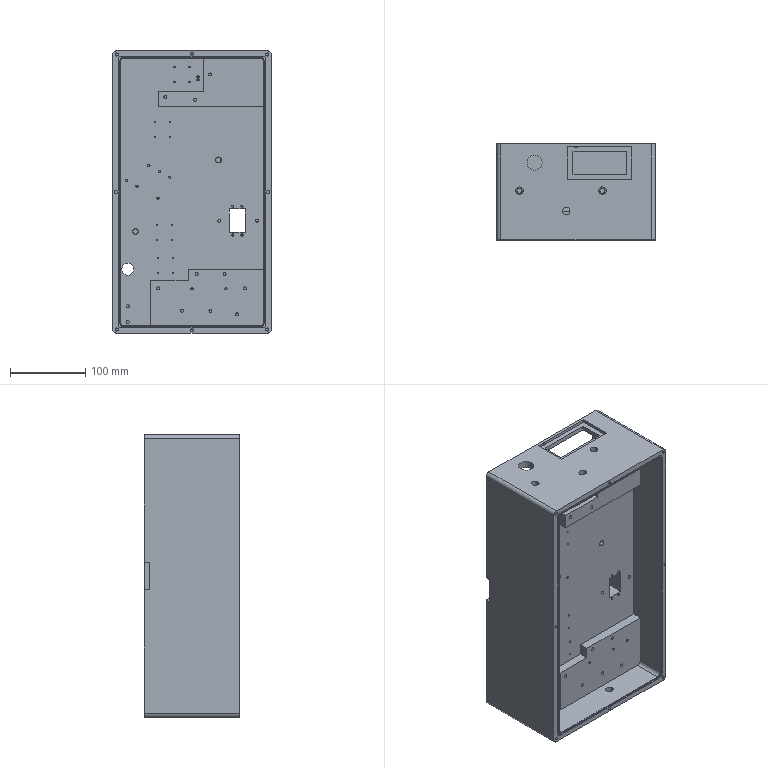Part | SolidWorks | features ICE 39, Fillet 6, MoveFace 4, Cut 3, Extrusion 1 | 1 solid | 361 faces | box 210 x 127 x 375 mm | volume 3262680 mm3 | cylinder 208 | plane 153 | commonest cylinder face diameters 4 x92 2 x36 3 x28 10 x28 7 x16 8 x4